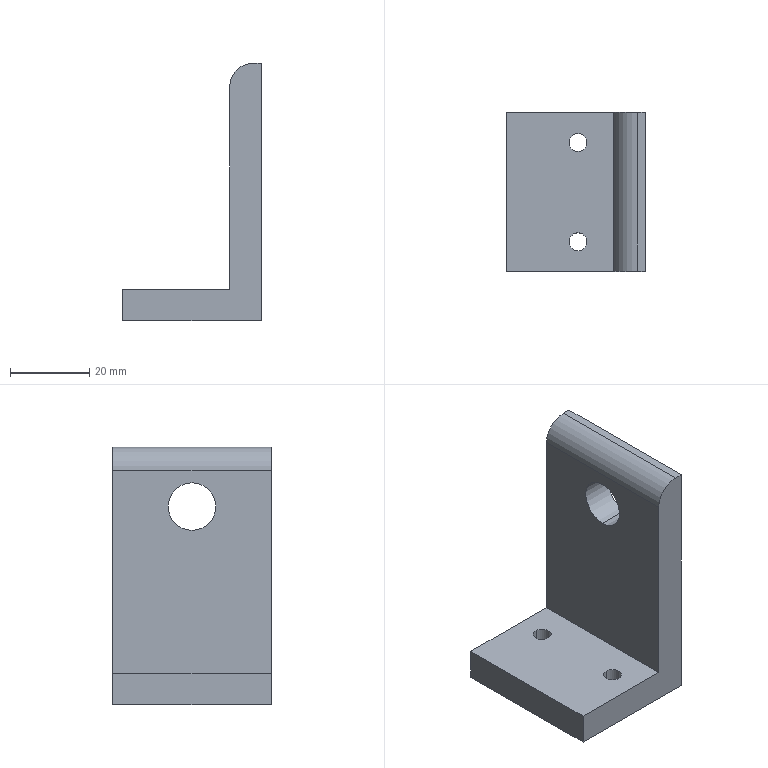Part | STEP file | Eyebolt mounting bracket-Part-1 | 1 solid | 15 faces | box 35 x 40 x 65 mm | volume 27972 mm3 | plane 8 | cylinder 7 | commonest cylinder face diameters 4.5 x4 12 x3
STEP:
#1=CARTESIAN_POINT('',(0.,0.,0.));
#2=DIRECTION('',(0.,0.,1.));
#3=DIRECTION('',(1.,0.,0.));
#4=AXIS2_PLACEMENT_3D('',#1,#2,#3);
#5=CARTESIAN_POINT('',(18.,5.25,8.));
#6=VERTEX_POINT('',#5);
#7=CARTESIAN_POINT('',(18.,5.25,0.));
#8=VERTEX_POINT('',#7);
#9=CARTESIAN_POINT('',(18.,5.25,8.));
#10=DIRECTION('',(0.,0.,-1.));
#11=VECTOR('',#10,1.);
#12=LINE('',#9,#11);
#13=CARTESIAN_POINT('',(18.,7.5,8.));
#14=DIRECTION('',(0.,0.,-1.));
#15=DIRECTION('',(0.,-1.,0.));
#16=AXIS2_PLACEMENT_3D('',#13,#14,#15);
#17=CYLINDRICAL_SURFACE('',#16,2.25);
#18=CARTESIAN_POINT('',(6.283,0.));
#19=DIRECTION('',(0.,1.));
#20=VECTOR('',#19,1.);
#21=LINE('',#18,#20);
#22=(GEOMETRIC_REPRESENTATION_CONTEXT(2)PARAMETRIC_REPRESENTATION_CONTEXT()REPRESENTATION_CONTEXT('',''));
#23=DEFINITIONAL_REPRESENTATION('',(#21),#22);
#24=PCURVE('',#17,#23);
#25=CARTESIAN_POINT('',(18.,7.5,8.));
#26=DIRECTION('',(0.,0.,-1.));
#27=DIRECTION('',(0.,-1.,0.));
#28=AXIS2_PLACEMENT_3D('',#25,#26,#27);
#29=CYLINDRICAL_SURFACE('',#28,2.25);
#30=CARTESIAN_POINT('',(0.,0.));
#31=DIRECTION('',(0.,1.));
#32=VECTOR('',#31,1.);
#33=LINE('',#30,#32);
#34=(GEOMETRIC_REPRESENTATION_CONTEXT(2)PARAMETRIC_REPRESENTATION_CONTEXT()REPRESENTATION_CONTEXT('',''));
#35=DEFINITIONAL_REPRESENTATION('',(#33),#34);
#36=PCURVE('',#29,#35);
#37=SURFACE_CURVE('',#12,(#24,#36),.PCURVE_S1.);
#38=EDGE_CURVE('',#6,#8,#37,.T.);
#39=ORIENTED_EDGE('',*,*,#38,.T.);
#40=CARTESIAN_POINT('',(18.,9.75,0.));
#41=VERTEX_POINT('',#40);
#42=CARTESIAN_POINT('',(18.,7.5,0.));
#43=DIRECTION('',(0.,0.,1.));
#44=DIRECTION('',(0.,1.,0.));
#45=AXIS2_PLACEMENT_3D('',#42,#43,#44);
#46=CIRCLE('',#45,2.25);
#47=CARTESIAN_POINT('',(9.425,8.));
#48=DIRECTION('',(-1.,0.));
#49=VECTOR('',#48,1.);
#50=LINE('',#47,#49);
#51=(GEOMETRIC_REPRESENTATION_CONTEXT(2)PARAMETRIC_REPRESENTATION_CONTEXT()REPRESENTATION_CONTEXT('',''));
#52=DEFINITIONAL_REPRESENTATION('',(#50),#51);
#53=PCURVE('',#17,#52);
#54=CARTESIAN_POINT('',(0.,0.,0.));
#55=DIRECTION('',(0.,0.,1.));
#56=DIRECTION('',(-1.,0.,0.));
#57=AXIS2_PLACEMENT_3D('',#54,#55,#56);
#58=PLANE('',#57);
#59=CARTESIAN_POINT('',(-18.,-7.5));
#60=DIRECTION('',(0.,-1.));
#61=AXIS2_PLACEMENT_2D('',#59,#60);
#62=CIRCLE('',#61,2.25);
#63=(GEOMETRIC_REPRESENTATION_CONTEXT(2)PARAMETRIC_REPRESENTATION_CONTEXT()REPRESENTATION_CONTEXT('',''));
#64=DEFINITIONAL_REPRESENTATION('',(#62),#63);
#65=PCURVE('',#58,#64);
#66=SURFACE_CURVE('',#46,(#53,#65),.PCURVE_S1.);
#67=EDGE_CURVE('',#8,#41,#66,.T.);
#68=ORIENTED_EDGE('',*,*,#67,.T.);
#69=CARTESIAN_POINT('',(18.,9.75,8.));
#70=VERTEX_POINT('',#69);
#71=CARTESIAN_POINT('',(18.,9.75,8.));
#72=DIRECTION('',(0.,0.,-1.));
#73=VECTOR('',#72,1.);
#74=LINE('',#71,#73);
#75=CARTESIAN_POINT('',(3.142,0.));
#76=DIRECTION('',(0.,1.));
#77=VECTOR('',#76,1.);
#78=LINE('',#75,#77);
#79=(GEOMETRIC_REPRESENTATION_CONTEXT(2)PARAMETRIC_REPRESENTATION_CONTEXT()REPRESENTATION_CONTEXT('',''));
#80=DEFINITIONAL_REPRESENTATION('',(#78),#79);
#81=PCURVE('',#17,#80);
#82=CARTESIAN_POINT('',(3.142,0.));
#83=DIRECTION('',(0.,1.));
#84=VECTOR('',#83,1.);
#85=LINE('',#82,#84);
#86=(GEOMETRIC_REPRESENTATION_CONTEXT(2)PARAMETRIC_REPRESENTATION_CONTEXT()REPRESENTATION_CONTEXT('',''));
#87=DEFINITIONAL_REPRESENTATION('',(#85),#86);
#88=PCURVE('',#29,#87);
#89=SURFACE_CURVE('',#74,(#81,#88),.PCURVE_S1.);
#90=EDGE_CURVE('',#70,#41,#89,.T.);
#91=ORIENTED_EDGE('',*,*,#90,.F.);
#92=CARTESIAN_POINT('',(18.,7.5,8.));
#93=DIRECTION('',(0.,0.,-1.));
#94=DIRECTION('',(0.,-1.,0.));
#95=AXIS2_PLACEMENT_3D('',#92,#93,#94);
#96=CIRCLE('',#95,2.25);
#97=CARTESIAN_POINT('',(0.,0.));
#98=DIRECTION('',(1.,0.));
#99=VECTOR('',#98,1.);
#100=LINE('',#97,#99);
#101=(GEOMETRIC_REPRESENTATION_CONTEXT(2)PARAMETRIC_REPRESENTATION_CONTEXT()REPRESENTATION_CONTEXT('',''));
#102=DEFINITIONAL_REPRESENTATION('',(#100),#101);
#103=PCURVE('',#17,#102);
#104=CARTESIAN_POINT('',(27.,0.,8.));
#105=DIRECTION('',(0.,0.,-1.));
#106=DIRECTION('',(1.,0.,0.));
#107=AXIS2_PLACEMENT_3D('',#104,#105,#106);
#108=PLANE('',#107);
#109=CARTESIAN_POINT('',(-9.,-7.5));
#110=DIRECTION('',(0.,1.));
#111=AXIS2_PLACEMENT_2D('',#109,#110);
#112=CIRCLE('',#111,2.25);
#113=(GEOMETRIC_REPRESENTATION_CONTEXT(2)PARAMETRIC_REPRESENTATION_CONTEXT()REPRESENTATION_CONTEXT('',''));
#114=DEFINITIONAL_REPRESENTATION('',(#112),#113);
#115=PCURVE('',#108,#114);
#116=SURFACE_CURVE('',#96,(#103,#115),.PCURVE_S1.);
#117=EDGE_CURVE('',#70,#6,#116,.T.);
#118=ORIENTED_EDGE('',*,*,#117,.T.);
#119=EDGE_LOOP('',(#39,#68,#91,#118));
#120=FACE_BOUND('',#119,.F.);
#121=ADVANCED_FACE('',(#120),#17,.F.);
#122=CARTESIAN_POINT('',(18.,30.25,8.));
#123=VERTEX_POINT('',#122);
#124=CARTESIAN_POINT('',(18.,30.25,0.));
#125=VERTEX_POINT('',#124);
#126=CARTESIAN_POINT('',(18.,30.25,8.));
#127=DIRECTION('',(0.,0.,-1.));
#128=VECTOR('',#127,1.);
#129=LINE('',#126,#128);
#130=CARTESIAN_POINT('',(18.,32.5,8.));
#131=DIRECTION('',(0.,0.,-1.));
#132=DIRECTION('',(0.,-1.,0.));
#133=AXIS2_PLACEMENT_3D('',#130,#131,#132);
#134=CYLINDRICAL_SURFACE('',#133,2.25);
#135=CARTESIAN_POINT('',(6.283,0.));
#136=DIRECTION('',(0.,1.));
#137=VECTOR('',#136,1.);
#138=LINE('',#135,#137);
#139=(GEOMETRIC_REPRESENTATION_CONTEXT(2)PARAMETRIC_REPRESENTATION_CONTEXT()REPRESENTATION_CONTEXT('',''));
#140=DEFINITIONAL_REPRESENTATION('',(#138),#139);
#141=PCURVE('',#134,#140);
#142=CARTESIAN_POINT('',(18.,32.5,8.));
#143=DIRECTION('',(0.,0.,-1.));
#144=DIRECTION('',(0.,-1.,0.));
#145=AXIS2_PLACEMENT_3D('',#142,#143,#144);
#146=CYLINDRICAL_SURFACE('',#145,2.25);
#147=CARTESIAN_POINT('',(0.,0.));
#148=DIRECTION('',(0.,1.));
#149=VECTOR('',#148,1.);
#150=LINE('',#147,#149);
#151=(GEOMETRIC_REPRESENTATION_CONTEXT(2)PARAMETRIC_REPRESENTATION_CONTEXT()REPRESENTATION_CONTEXT('',''));
#152=DEFINITIONAL_REPRESENTATION('',(#150),#151);
#153=PCURVE('',#146,#152);
#154=SURFACE_CURVE('',#129,(#141,#153),.PCURVE_S1.);
#155=EDGE_CURVE('',#123,#125,#154,.T.);
#156=ORIENTED_EDGE('',*,*,#155,.T.);
#157=CARTESIAN_POINT('',(18.,34.75,0.));
#158=VERTEX_POINT('',#157);
#159=CARTESIAN_POINT('',(18.,32.5,0.));
#160=DIRECTION('',(0.,0.,1.));
#161=DIRECTION('',(0.,1.,0.));
#162=AXIS2_PLACEMENT_3D('',#159,#160,#161);
#163=CIRCLE('',#162,2.25);
#164=CARTESIAN_POINT('',(9.425,8.));
#165=DIRECTION('',(-1.,0.));
#166=VECTOR('',#165,1.);
#167=LINE('',#164,#166);
#168=(GEOMETRIC_REPRESENTATION_CONTEXT(2)PARAMETRIC_REPRESENTATION_CONTEXT()REPRESENTATION_CONTEXT('',''));
#169=DEFINITIONAL_REPRESENTATION('',(#167),#168);
#170=PCURVE('',#134,#169);
#171=CARTESIAN_POINT('',(-18.,-32.5));
#172=DIRECTION('',(0.,-1.));
#173=AXIS2_PLACEMENT_2D('',#171,#172);
#174=CIRCLE('',#173,2.25);
#175=(GEOMETRIC_REPRESENTATION_CONTEXT(2)PARAMETRIC_REPRESENTATION_CONTEXT()REPRESENTATION_CONTEXT('',''));
#176=DEFINITIONAL_REPRESENTATION('',(#174),#175);
#177=PCURVE('',#58,#176);
#178=SURFACE_CURVE('',#163,(#170,#177),.PCURVE_S1.);
#179=EDGE_CURVE('',#125,#158,#178,.T.);
#180=ORIENTED_EDGE('',*,*,#179,.T.);
#181=CARTESIAN_POINT('',(18.,34.75,8.));
#182=VERTEX_POINT('',#181);
#183=CARTESIAN_POINT('',(18.,34.75,8.));
#184=DIRECTION('',(0.,0.,-1.));
#185=VECTOR('',#184,1.);
#186=LINE('',#183,#185);
#187=CARTESIAN_POINT('',(3.142,0.));
#188=DIRECTION('',(0.,1.));
#189=VECTOR('',#188,1.);
#190=LINE('',#187,#189);
#191=(GEOMETRIC_REPRESENTATION_CONTEXT(2)PARAMETRIC_REPRESENTATION_CONTEXT()REPRESENTATION_CONTEXT('',''));
#192=DEFINITIONAL_REPRESENTATION('',(#190),#191);
#193=PCURVE('',#134,#192);
#194=CARTESIAN_POINT('',(3.142,0.));
#195=DIRECTION('',(0.,1.));
#196=VECTOR('',#195,1.);
#197=LINE('',#194,#196);
#198=(GEOMETRIC_REPRESENTATION_CONTEXT(2)PARAMETRIC_REPRESENTATION_CONTEXT()REPRESENTATION_CONTEXT('',''));
#199=DEFINITIONAL_REPRESENTATION('',(#197),#198);
#200=PCURVE('',#146,#199);
#201=SURFACE_CURVE('',#186,(#193,#200),.PCURVE_S1.);
#202=EDGE_CURVE('',#182,#158,#201,.T.);
#203=ORIENTED_EDGE('',*,*,#202,.F.);
#204=CARTESIAN_POINT('',(18.,32.5,8.));
#205=DIRECTION('',(0.,0.,-1.));
#206=DIRECTION('',(0.,-1.,0.));
#207=AXIS2_PLACEMENT_3D('',#204,#205,#206);
#208=CIRCLE('',#207,2.25);
#209=CARTESIAN_POINT('',(0.,0.));
#210=DIRECTION('',(1.,0.));
#211=VECTOR('',#210,1.);
#212=LINE('',#209,#211);
#213=(GEOMETRIC_REPRESENTATION_CONTEXT(2)PARAMETRIC_REPRESENTATION_CONTEXT()REPRESENTATION_CONTEXT('',''));
#214=DEFINITIONAL_REPRESENTATION('',(#212),#213);
#215=PCURVE('',#134,#214);
#216=CARTESIAN_POINT('',(-9.,-32.5));
#217=DIRECTION('',(0.,1.));
#218=AXIS2_PLACEMENT_2D('',#216,#217);
#219=CIRCLE('',#218,2.25);
#220=(GEOMETRIC_REPRESENTATION_CONTEXT(2)PARAMETRIC_REPRESENTATION_CONTEXT()REPRESENTATION_CONTEXT('',''));
#221=DEFINITIONAL_REPRESENTATION('',(#219),#220);
#222=PCURVE('',#108,#221);
#223=SURFACE_CURVE('',#208,(#215,#222),.PCURVE_S1.);
#224=EDGE_CURVE('',#182,#123,#223,.T.);
#225=ORIENTED_EDGE('',*,*,#224,.T.);
#226=EDGE_LOOP('',(#156,#180,#203,#225));
#227=FACE_BOUND('',#226,.F.);
#228=ADVANCED_FACE('',(#227),#134,.F.);
#229=CARTESIAN_POINT('',(35.,20.,44.));
#230=VERTEX_POINT('',#229);
#231=CARTESIAN_POINT('',(27.,20.,44.));
#232=VERTEX_POINT('',#231);
#233=CARTESIAN_POINT('',(35.,20.,44.));
#234=DIRECTION('',(-1.,0.,0.));
#235=VECTOR('',#234,1.);
#236=LINE('',#233,#235);
#237=CARTESIAN_POINT('',(35.,20.,50.));
#238=DIRECTION('',(-1.,0.,0.));
#239=DIRECTION('',(0.,0.,-1.));
#240=AXIS2_PLACEMENT_3D('',#237,#238,#239);
#241=CYLINDRICAL_SURFACE('',#240,6.);
#242=CARTESIAN_POINT('',(6.283,0.));
#243=DIRECTION('',(0.,1.));
#244=VECTOR('',#243,1.);
#245=LINE('',#242,#244);
#246=(GEOMETRIC_REPRESENTATION_CONTEXT(2)PARAMETRIC_REPRESENTATION_CONTEXT()REPRESENTATION_CONTEXT('',''));
#247=DEFINITIONAL_REPRESENTATION('',(#245),#246);
#248=PCURVE('',#241,#247);
#249=CARTESIAN_POINT('',(35.,20.,50.));
#250=DIRECTION('',(-1.,0.,0.));
#251=DIRECTION('',(0.,0.,-1.));
#252=AXIS2_PLACEMENT_3D('',#249,#250,#251);
#253=CYLINDRICAL_SURFACE('',#252,6.);
#254=CARTESIAN_POINT('',(0.,0.));
#255=DIRECTION('',(0.,1.));
#256=VECTOR('',#255,1.);
#257=LINE('',#254,#256);
#258=(GEOMETRIC_REPRESENTATION_CONTEXT(2)PARAMETRIC_REPRESENTATION_CONTEXT()REPRESENTATION_CONTEXT('',''));
#259=DEFINITIONAL_REPRESENTATION('',(#257),#258);
#260=PCURVE('',#253,#259);
#261=SURFACE_CURVE('',#236,(#248,#260),.PCURVE_S1.);
#262=EDGE_CURVE('',#230,#232,#261,.T.);
#263=ORIENTED_EDGE('',*,*,#262,.T.);
#264=CARTESIAN_POINT('',(27.,20.,56.));
#265=VERTEX_POINT('',#264);
#266=CARTESIAN_POINT('',(27.,20.,50.));
#267=DIRECTION('',(1.,0.,0.));
#268=DIRECTION('',(0.,0.,1.));
#269=AXIS2_PLACEMENT_3D('',#266,#267,#268);
#270=CIRCLE('',#269,6.);
#271=CARTESIAN_POINT('',(9.425,8.));
#272=DIRECTION('',(-1.,0.));
#273=VECTOR('',#272,1.);
#274=LINE('',#271,#273);
#275=(GEOMETRIC_REPRESENTATION_CONTEXT(2)PARAMETRIC_REPRESENTATION_CONTEXT()REPRESENTATION_CONTEXT('',''));
#276=DEFINITIONAL_REPRESENTATION('',(#274),#275);
#277=PCURVE('',#241,#276);
#278=CARTESIAN_POINT('',(27.,0.,59.));
#279=DIRECTION('',(1.,0.,0.));
#280=DIRECTION('',(0.,0.,1.));
#281=AXIS2_PLACEMENT_3D('',#278,#279,#280);
#282=PLANE('',#281);
#283=CARTESIAN_POINT('',(-9.,-20.));
#284=DIRECTION('',(1.,0.));
#285=AXIS2_PLACEMENT_2D('',#283,#284);
#286=CIRCLE('',#285,6.);
#287=(GEOMETRIC_REPRESENTATION_CONTEXT(2)PARAMETRIC_REPRESENTATION_CONTEXT()REPRESENTATION_CONTEXT('',''));
#288=DEFINITIONAL_REPRESENTATION('',(#286),#287);
#289=PCURVE('',#282,#288);
#290=SURFACE_CURVE('',#270,(#277,#289),.PCURVE_S1.);
#291=EDGE_CURVE('',#232,#265,#290,.T.);
#292=ORIENTED_EDGE('',*,*,#291,.T.);
#293=CARTESIAN_POINT('',(35.,20.,56.));
#294=VERTEX_POINT('',#293);
#295=CARTESIAN_POINT('',(35.,20.,56.));
#296=DIRECTION('',(-1.,0.,0.));
#297=VECTOR('',#296,1.);
#298=LINE('',#295,#297);
#299=CARTESIAN_POINT('',(3.142,0.));
#300=DIRECTION('',(0.,1.));
#301=VECTOR('',#300,1.);
#302=LINE('',#299,#301);
#303=(GEOMETRIC_REPRESENTATION_CONTEXT(2)PARAMETRIC_REPRESENTATION_CONTEXT()REPRESENTATION_CONTEXT('',''));
#304=DEFINITIONAL_REPRESENTATION('',(#302),#303);
#305=PCURVE('',#241,#304);
#306=CARTESIAN_POINT('',(3.142,0.));
#307=DIRECTION('',(0.,1.));
#308=VECTOR('',#307,1.);
#309=LINE('',#306,#308);
#310=(GEOMETRIC_REPRESENTATION_CONTEXT(2)PARAMETRIC_REPRESENTATION_CONTEXT()REPRESENTATION_CONTEXT('',''));
#311=DEFINITIONAL_REPRESENTATION('',(#309),#310);
#312=PCURVE('',#253,#311);
#313=SURFACE_CURVE('',#298,(#305,#312),.PCURVE_S1.);
#314=EDGE_CURVE('',#294,#265,#313,.T.);
#315=ORIENTED_EDGE('',*,*,#314,.F.);
#316=CARTESIAN_POINT('',(35.,20.,50.));
#317=DIRECTION('',(-1.,0.,0.));
#318=DIRECTION('',(0.,0.,-1.));
#319=AXIS2_PLACEMENT_3D('',#316,#317,#318);
#320=CIRCLE('',#319,6.);
#321=CARTESIAN_POINT('',(0.,0.));
#322=DIRECTION('',(1.,0.));
#323=VECTOR('',#322,1.);
#324=LINE('',#321,#323);
#325=(GEOMETRIC_REPRESENTATION_CONTEXT(2)PARAMETRIC_REPRESENTATION_CONTEXT()REPRESENTATION_CONTEXT('',''));
#326=DEFINITIONAL_REPRESENTATION('',(#324),#325);
#327=PCURVE('',#241,#326);
#328=CARTESIAN_POINT('',(35.,0.,0.));
#329=DIRECTION('',(-1.,0.,0.));
#330=DIRECTION('',(0.,0.,-1.));
#331=AXIS2_PLACEMENT_3D('',#328,#329,#330);
#332=PLANE('',#331);
#333=CARTESIAN_POINT('',(-50.,-20.));
#334=DIRECTION('',(1.,0.));
#335=AXIS2_PLACEMENT_2D('',#333,#334);
#336=CIRCLE('',#335,6.);
#337=(GEOMETRIC_REPRESENTATION_CONTEXT(2)PARAMETRIC_REPRESENTATION_CONTEXT()REPRESENTATION_CONTEXT('',''));
#338=DEFINITIONAL_REPRESENTATION('',(#336),#337);
#339=PCURVE('',#332,#338);
#340=SURFACE_CURVE('',#320,(#327,#339),.PCURVE_S1.);
#341=EDGE_CURVE('',#294,#230,#340,.T.);
#342=ORIENTED_EDGE('',*,*,#341,.T.);
#343=EDGE_LOOP('',(#263,#292,#315,#342));
#344=FACE_BOUND('',#343,.F.);
#345=ADVANCED_FACE('',(#344),#241,.F.);
#346=ORIENTED_EDGE('',*,*,#67,.T.);
#347=CARTESIAN_POINT('',(18.,7.5,0.));
#348=DIRECTION('',(0.,0.,1.));
#349=DIRECTION('',(0.,1.,0.));
#350=AXIS2_PLACEMENT_3D('',#347,#348,#349);
#351=CIRCLE('',#350,2.25);
#352=CARTESIAN_POINT('',(-18.,-7.5));
#353=DIRECTION('',(0.,-1.));
#354=AXIS2_PLACEMENT_2D('',#352,#353);
#355=CIRCLE('',#354,2.25);
#356=(GEOMETRIC_REPRESENTATION_CONTEXT(2)PARAMETRIC_REPRESENTATION_CONTEXT()REPRESENTATION_CONTEXT('',''));
#357=DEFINITIONAL_REPRESENTATION('',(#355),#356);
#358=PCURVE('',#58,#357);
#359=CARTESIAN_POINT('',(3.142,8.));
#360=DIRECTION('',(-1.,0.));
#361=VECTOR('',#360,1.);
#362=LINE('',#359,#361);
#363=(GEOMETRIC_REPRESENTATION_CONTEXT(2)PARAMETRIC_REPRESENTATION_CONTEXT()REPRESENTATION_CONTEXT('',''));
#364=DEFINITIONAL_REPRESENTATION('',(#362),#363);
#365=PCURVE('',#29,#364);
#366=SURFACE_CURVE('',#351,(#358,#365),.PCURVE_S1.);
#367=EDGE_CURVE('',#41,#8,#366,.T.);
#368=ORIENTED_EDGE('',*,*,#367,.T.);
#369=EDGE_LOOP('',(#346,#368));
#370=FACE_BOUND('',#369,.T.);
#371=ORIENTED_EDGE('',*,*,#179,.T.);
#372=CARTESIAN_POINT('',(18.,32.5,0.));
#373=DIRECTION('',(0.,0.,1.));
#374=DIRECTION('',(0.,1.,0.));
#375=AXIS2_PLACEMENT_3D('',#372,#373,#374);
#376=CIRCLE('',#375,2.25);
#377=CARTESIAN_POINT('',(-18.,-32.5));
#378=DIRECTION('',(0.,-1.));
#379=AXIS2_PLACEMENT_2D('',#377,#378);
#380=CIRCLE('',#379,2.25);
#381=(GEOMETRIC_REPRESENTATION_CONTEXT(2)PARAMETRIC_REPRESENTATION_CONTEXT()REPRESENTATION_CONTEXT('',''));
#382=DEFINITIONAL_REPRESENTATION('',(#380),#381);
#383=PCURVE('',#58,#382);
#384=CARTESIAN_POINT('',(3.142,8.));
#385=DIRECTION('',(-1.,0.));
#386=VECTOR('',#385,1.);
#387=LINE('',#384,#386);
#388=(GEOMETRIC_REPRESENTATION_CONTEXT(2)PARAMETRIC_REPRESENTATION_CONTEXT()REPRESENTATION_CONTEXT('',''));
#389=DEFINITIONAL_REPRESENTATION('',(#387),#388);
#390=PCURVE('',#146,#389);
#391=SURFACE_CURVE('',#376,(#383,#390),.PCURVE_S1.);
#392=EDGE_CURVE('',#158,#125,#391,.T.);
#393=ORIENTED_EDGE('',*,*,#392,.T.);
#394=EDGE_LOOP('',(#371,#393));
#395=FACE_BOUND('',#394,.T.);
#396=CARTESIAN_POINT('',(0.,40.,0.));
#397=VERTEX_POINT('',#396);
#398=CARTESIAN_POINT('',(35.,40.,0.));
#399=VERTEX_POINT('',#398);
#400=CARTESIAN_POINT('',(0.,40.,0.));
#401=DIRECTION('',(1.,0.,0.));
#402=VECTOR('',#401,1.);
#403=LINE('',#400,#402);
#404=CARTESIAN_POINT('',(0.,-40.));
#405=DIRECTION('',(-1.,0.));
#406=VECTOR('',#405,1.);
#407=LINE('',#404,#406);
#408=(GEOMETRIC_REPRESENTATION_CONTEXT(2)PARAMETRIC_REPRESENTATION_CONTEXT()REPRESENTATION_CONTEXT('',''));
#409=DEFINITIONAL_REPRESENTATION('',(#407),#408);
#410=PCURVE('',#58,#409);
#411=CARTESIAN_POINT('',(33.,40.,59.));
#412=DIRECTION('',(0.,-1.,0.));
#413=DIRECTION('',(0.,0.,1.));
#414=AXIS2_PLACEMENT_3D('',#411,#412,#413);
#415=PLANE('',#414);
#416=CARTESIAN_POINT('',(-59.,33.));
#417=DIRECTION('',(0.,-1.));
#418=VECTOR('',#417,1.);
#419=LINE('',#416,#418);
#420=(GEOMETRIC_REPRESENTATION_CONTEXT(2)PARAMETRIC_REPRESENTATION_CONTEXT()REPRESENTATION_CONTEXT('',''));
#421=DEFINITIONAL_REPRESENTATION('',(#419),#420);
#422=PCURVE('',#415,#421);
#423=SURFACE_CURVE('',#403,(#410,#422),.PCURVE_S1.);
#424=EDGE_CURVE('',#397,#399,#423,.T.);
#425=ORIENTED_EDGE('',*,*,#424,.T.);
#426=CARTESIAN_POINT('',(35.,0.,0.));
#427=VERTEX_POINT('',#426);
#428=CARTESIAN_POINT('',(35.,0.,0.));
#429=DIRECTION('',(0.,1.,0.));
#430=VECTOR('',#429,1.);
#431=LINE('',#428,#430);
#432=CARTESIAN_POINT('',(-35.,0.));
#433=DIRECTION('',(0.,-1.));
#434=VECTOR('',#433,1.);
#435=LINE('',#432,#434);
#436=(GEOMETRIC_REPRESENTATION_CONTEXT(2)PARAMETRIC_REPRESENTATION_CONTEXT()REPRESENTATION_CONTEXT('',''));
#437=DEFINITIONAL_REPRESENTATION('',(#435),#436);
#438=PCURVE('',#58,#437);
#439=CARTESIAN_POINT('',(0.,0.));
#440=DIRECTION('',(0.,-1.));
#441=VECTOR('',#440,1.);
#442=LINE('',#439,#441);
#443=(GEOMETRIC_REPRESENTATION_CONTEXT(2)PARAMETRIC_REPRESENTATION_CONTEXT()REPRESENTATION_CONTEXT('',''));
#444=DEFINITIONAL_REPRESENTATION('',(#442),#443);
#445=PCURVE('',#332,#444);
#446=SURFACE_CURVE('',#431,(#438,#445),.PCURVE_S1.);
#447=EDGE_CURVE('',#427,#399,#446,.T.);
#448=ORIENTED_EDGE('',*,*,#447,.F.);
#449=CARTESIAN_POINT('',(0.,0.,0.));
#450=VERTEX_POINT('',#449);
#451=CARTESIAN_POINT('',(0.,0.,0.));
#452=DIRECTION('',(1.,0.,0.));
#453=VECTOR('',#452,1.);
#454=LINE('',#451,#453);
#455=CARTESIAN_POINT('',(0.,0.));
#456=DIRECTION('',(-1.,0.));
#457=VECTOR('',#456,1.);
#458=LINE('',#455,#457);
#459=(GEOMETRIC_REPRESENTATION_CONTEXT(2)PARAMETRIC_REPRESENTATION_CONTEXT()REPRESENTATION_CONTEXT('',''));
#460=DEFINITIONAL_REPRESENTATION('',(#458),#459);
#461=PCURVE('',#58,#460);
#462=CARTESIAN_POINT('',(33.,0.,59.));
#463=DIRECTION('',(0.,-1.,0.));
#464=DIRECTION('',(0.,0.,1.));
#465=AXIS2_PLACEMENT_3D('',#462,#463,#464);
#466=PLANE('',#465);
#467=CARTESIAN_POINT('',(-59.,33.));
#468=DIRECTION('',(0.,-1.));
#469=VECTOR('',#468,1.);
#470=LINE('',#467,#469);
#471=(GEOMETRIC_REPRESENTATION_CONTEXT(2)PARAMETRIC_REPRESENTATION_CONTEXT()REPRESENTATION_CONTEXT('',''));
#472=DEFINITIONAL_REPRESENTATION('',(#470),#471);
#473=PCURVE('',#466,#472);
#474=SURFACE_CURVE('',#454,(#461,#473),.PCURVE_S1.);
#475=EDGE_CURVE('',#450,#427,#474,.T.);
#476=ORIENTED_EDGE('',*,*,#475,.F.);
#477=CARTESIAN_POINT('',(0.,0.,0.));
#478=DIRECTION('',(0.,1.,0.));
#479=VECTOR('',#478,1.);
#480=LINE('',#477,#479);
#481=CARTESIAN_POINT('',(0.,0.));
#482=DIRECTION('',(0.,-1.));
#483=VECTOR('',#482,1.);
#484=LINE('',#481,#483);
#485=(GEOMETRIC_REPRESENTATION_CONTEXT(2)PARAMETRIC_REPRESENTATION_CONTEXT()REPRESENTATION_CONTEXT('',''));
#486=DEFINITIONAL_REPRESENTATION('',(#484),#485);
#487=PCURVE('',#58,#486);
#488=CARTESIAN_POINT('',(0.,0.,8.));
#489=DIRECTION('',(1.,0.,0.));
#490=DIRECTION('',(0.,1.,0.));
#491=AXIS2_PLACEMENT_3D('',#488,#489,#490);
#492=PLANE('',#491);
#493=CARTESIAN_POINT('',(0.,-8.));
#494=DIRECTION('',(1.,0.));
#495=VECTOR('',#494,1.);
#496=LINE('',#493,#495);
#497=(GEOMETRIC_REPRESENTATION_CONTEXT(2)PARAMETRIC_REPRESENTATION_CONTEXT()REPRESENTATION_CONTEXT('',''));
#498=DEFINITIONAL_REPRESENTATION('',(#496),#497);
#499=PCURVE('',#492,#498);
#500=SURFACE_CURVE('',#480,(#487,#499),.PCURVE_S1.);
#501=EDGE_CURVE('',#450,#397,#500,.T.);
#502=ORIENTED_EDGE('',*,*,#501,.T.);
#503=EDGE_LOOP('',(#425,#448,#476,#502));
#504=FACE_BOUND('',#503,.T.);
#505=ADVANCED_FACE('',(#370,#395,#504),#58,.F.);
#506=CARTESIAN_POINT('',(35.,20.,50.));
#507=DIRECTION('',(-1.,0.,0.));
#508=DIRECTION('',(0.,0.,-1.));
#509=AXIS2_PLACEMENT_3D('',#506,#507,#508);
#510=CIRCLE('',#509,6.);
#511=CARTESIAN_POINT('',(-50.,-20.));
#512=DIRECTION('',(1.,0.));
#513=AXIS2_PLACEMENT_2D('',#511,#512);
#514=CIRCLE('',#513,6.);
#515=(GEOMETRIC_REPRESENTATION_CONTEXT(2)PARAMETRIC_REPRESENTATION_CONTEXT()REPRESENTATION_CONTEXT('',''));
#516=DEFINITIONAL_REPRESENTATION('',(#514),#515);
#517=PCURVE('',#332,#516);
#518=CARTESIAN_POINT('',(0.,0.));
#519=DIRECTION('',(1.,0.));
#520=VECTOR('',#519,1.);
#521=LINE('',#518,#520);
#522=(GEOMETRIC_REPRESENTATION_CONTEXT(2)PARAMETRIC_REPRESENTATION_CONTEXT()REPRESENTATION_CONTEXT('',''));
#523=DEFINITIONAL_REPRESENTATION('',(#521),#522);
#524=PCURVE('',#253,#523);
#525=SURFACE_CURVE('',#510,(#517,#524),.PCURVE_S1.);
#526=EDGE_CURVE('',#230,#294,#525,.T.);
#527=ORIENTED_EDGE('',*,*,#526,.T.);
#528=ORIENTED_EDGE('',*,*,#341,.T.);
#529=EDGE_LOOP('',(#527,#528));
#530=FACE_BOUND('',#529,.T.);
#531=CARTESIAN_POINT('',(35.,40.,65.));
#532=VERTEX_POINT('',#531);
#533=CARTESIAN_POINT('',(35.,40.,0.));
#534=DIRECTION('',(0.,0.,1.));
#535=VECTOR('',#534,1.);
#536=LINE('',#533,#535);
#537=CARTESIAN_POINT('',(0.,-40.));
#538=DIRECTION('',(-1.,0.));
#539=VECTOR('',#538,1.);
#540=LINE('',#537,#539);
#541=(GEOMETRIC_REPRESENTATION_CONTEXT(2)PARAMETRIC_REPRESENTATION_CONTEXT()REPRESENTATION_CONTEXT('',''));
#542=DEFINITIONAL_REPRESENTATION('',(#540),#541);
#543=PCURVE('',#332,#542);
#544=CARTESIAN_POINT('',(-59.,-2.));
#545=DIRECTION('',(1.,0.));
#546=VECTOR('',#545,1.);
#547=LINE('',#544,#546);
#548=(GEOMETRIC_REPRESENTATION_CONTEXT(2)PARAMETRIC_REPRESENTATION_CONTEXT()REPRESENTATION_CONTEXT('',''));
#549=DEFINITIONAL_REPRESENTATION('',(#547),#548);
#550=PCURVE('',#415,#549);
#551=SURFACE_CURVE('',#536,(#543,#550),.PCURVE_S1.);
#552=EDGE_CURVE('',#399,#532,#551,.T.);
#553=ORIENTED_EDGE('',*,*,#552,.T.);
#554=CARTESIAN_POINT('',(35.,0.,65.));
#555=VERTEX_POINT('',#554);
#556=CARTESIAN_POINT('',(35.,0.,65.));
#557=DIRECTION('',(0.,1.,0.));
#558=VECTOR('',#557,1.);
#559=LINE('',#556,#558);
#560=CARTESIAN_POINT('',(-65.,0.));
#561=DIRECTION('',(0.,-1.));
#562=VECTOR('',#561,1.);
#563=LINE('',#560,#562);
#564=(GEOMETRIC_REPRESENTATION_CONTEXT(2)PARAMETRIC_REPRESENTATION_CONTEXT()REPRESENTATION_CONTEXT('',''));
#565=DEFINITIONAL_REPRESENTATION('',(#563),#564);
#566=PCURVE('',#332,#565);
#567=CARTESIAN_POINT('',(35.,0.,65.));
#568=DIRECTION('',(0.,0.,-1.));
#569=DIRECTION('',(0.,-1.,0.));
#570=AXIS2_PLACEMENT_3D('',#567,#568,#569);
#571=PLANE('',#570);
#572=CARTESIAN_POINT('',(0.,0.));
#573=DIRECTION('',(-1.,0.));
#574=VECTOR('',#573,1.);
#575=LINE('',#572,#574);
#576=(GEOMETRIC_REPRESENTATION_CONTEXT(2)PARAMETRIC_REPRESENTATION_CONTEXT()REPRESENTATION_CONTEXT('',''));
#577=DEFINITIONAL_REPRESENTATION('',(#575),#576);
#578=PCURVE('',#571,#577);
#579=SURFACE_CURVE('',#559,(#566,#578),.PCURVE_S1.);
#580=EDGE_CURVE('',#555,#532,#579,.T.);
#581=ORIENTED_EDGE('',*,*,#580,.F.);
#582=CARTESIAN_POINT('',(35.,0.,0.));
#583=DIRECTION('',(0.,0.,1.));
#584=VECTOR('',#583,1.);
#585=LINE('',#582,#584);
#586=CARTESIAN_POINT('',(0.,0.));
#587=DIRECTION('',(-1.,0.));
#588=VECTOR('',#587,1.);
#589=LINE('',#586,#588);
#590=(GEOMETRIC_REPRESENTATION_CONTEXT(2)PARAMETRIC_REPRESENTATION_CONTEXT()REPRESENTATION_CONTEXT('',''));
#591=DEFINITIONAL_REPRESENTATION('',(#589),#590);
#592=PCURVE('',#332,#591);
#593=CARTESIAN_POINT('',(-59.,-2.));
#594=DIRECTION('',(1.,0.));
#595=VECTOR('',#594,1.);
#596=LINE('',#593,#595);
#597=(GEOMETRIC_REPRESENTATION_CONTEXT(2)PARAMETRIC_REPRESENTATION_CONTEXT()REPRESENTATION_CONTEXT('',''));
#598=DEFINITIONAL_REPRESENTATION('',(#596),#597);
#599=PCURVE('',#466,#598);
#600=SURFACE_CURVE('',#585,(#592,#599),.PCURVE_S1.);
#601=EDGE_CURVE('',#427,#555,#600,.T.);
#602=ORIENTED_EDGE('',*,*,#601,.F.);
#603=ORIENTED_EDGE('',*,*,#447,.T.);
#604=EDGE_LOOP('',(#553,#581,#602,#603));
#605=FACE_BOUND('',#604,.T.);
#606=ADVANCED_FACE('',(#530,#605),#332,.F.);
#607=CARTESIAN_POINT('',(33.,40.,65.));
#608=VERTEX_POINT('',#607);
#609=CARTESIAN_POINT('',(35.,40.,65.));
#610=DIRECTION('',(-1.,0.,0.));
#611=VECTOR('',#610,1.);
#612=LINE('',#609,#611);
#613=CARTESIAN_POINT('',(-40.,0.));
#614=DIRECTION('',(0.,1.));
#615=VECTOR('',#614,1.);
#616=LINE('',#613,#615);
#617=(GEOMETRIC_REPRESENTATION_CONTEXT(2)PARAMETRIC_REPRESENTATION_CONTEXT()REPRESENTATION_CONTEXT('',''));
#618=DEFINITIONAL_REPRESENTATION('',(#616),#617);
#619=PCURVE('',#571,#618);
#620=CARTESIAN_POINT('',(6.,-2.));
#621=DIRECTION('',(0.,1.));
#622=VECTOR('',#621,1.);
#623=LINE('',#620,#622);
#624=(GEOMETRIC_REPRESENTATION_CONTEXT(2)PARAMETRIC_REPRESENTATION_CONTEXT()REPRESENTATION_CONTEXT('',''));
#625=DEFINITIONAL_REPRESENTATION('',(#623),#624);
#626=PCURVE('',#415,#625);
#627=SURFACE_CURVE('',#612,(#619,#626),.PCURVE_S1.);
#628=EDGE_CURVE('',#532,#608,#627,.T.);
#629=ORIENTED_EDGE('',*,*,#628,.T.);
#630=CARTESIAN_POINT('',(33.,0.,65.));
#631=VERTEX_POINT('',#630);
#632=CARTESIAN_POINT('',(33.,0.,65.));
#633=DIRECTION('',(0.,1.,0.));
#634=VECTOR('',#633,1.);
#635=LINE('',#632,#634);
#636=CARTESIAN_POINT('',(0.,2.));
#637=DIRECTION('',(-1.,0.));
#638=VECTOR('',#637,1.);
#639=LINE('',#636,#638);
#640=(GEOMETRIC_REPRESENTATION_CONTEXT(2)PARAMETRIC_REPRESENTATION_CONTEXT()REPRESENTATION_CONTEXT('',''));
#641=DEFINITIONAL_REPRESENTATION('',(#639),#640);
#642=PCURVE('',#571,#641);
#643=CARTESIAN_POINT('',(33.,0.,59.));
#644=DIRECTION('',(0.,1.,0.));
#645=DIRECTION('',(0.,0.,-1.));
#646=AXIS2_PLACEMENT_3D('',#643,#644,#645);
#647=CYLINDRICAL_SURFACE('',#646,6.);
#648=CARTESIAN_POINT('',(3.142,0.));
#649=DIRECTION('',(0.,1.));
#650=VECTOR('',#649,1.);
#651=LINE('',#648,#650);
#652=(GEOMETRIC_REPRESENTATION_CONTEXT(2)PARAMETRIC_REPRESENTATION_CONTEXT()REPRESENTATION_CONTEXT('',''));
#653=DEFINITIONAL_REPRESENTATION('',(#651),#652);
#654=PCURVE('',#647,#653);
#655=SURFACE_CURVE('',#635,(#642,#654),.PCURVE_S1.);
#656=EDGE_CURVE('',#631,#608,#655,.T.);
#657=ORIENTED_EDGE('',*,*,#656,.F.);
#658=CARTESIAN_POINT('',(35.,0.,65.));
#659=DIRECTION('',(-1.,0.,0.));
#660=VECTOR('',#659,1.);
#661=LINE('',#658,#660);
#662=CARTESIAN_POINT('',(0.,0.));
#663=DIRECTION('',(0.,1.));
#664=VECTOR('',#663,1.);
#665=LINE('',#662,#664);
#666=(GEOMETRIC_REPRESENTATION_CONTEXT(2)PARAMETRIC_REPRESENTATION_CONTEXT()REPRESENTATION_CONTEXT('',''));
#667=DEFINITIONAL_REPRESENTATION('',(#665),#666);
#668=PCURVE('',#571,#667);
#669=CARTESIAN_POINT('',(6.,-2.));
#670=DIRECTION('',(0.,1.));
#671=VECTOR('',#670,1.);
#672=LINE('',#669,#671);
#673=(GEOMETRIC_REPRESENTATION_CONTEXT(2)PARAMETRIC_REPRESENTATION_CONTEXT()REPRESENTATION_CONTEXT('',''));
#674=DEFINITIONAL_REPRESENTATION('',(#672),#673);
#675=PCURVE('',#466,#674);
#676=SURFACE_CURVE('',#661,(#668,#675),.PCURVE_S1.);
#677=EDGE_CURVE('',#555,#631,#676,.T.);
#678=ORIENTED_EDGE('',*,*,#677,.F.);
#679=ORIENTED_EDGE('',*,*,#580,.T.);
#680=EDGE_LOOP('',(#629,#657,#678,#679));
#681=FACE_BOUND('',#680,.T.);
#682=ADVANCED_FACE('',(#681),#571,.F.);
#683=CARTESIAN_POINT('',(27.,40.,59.));
#684=VERTEX_POINT('',#683);
#685=CARTESIAN_POINT('',(33.,40.,59.));
#686=DIRECTION('',(0.,-1.,0.));
#687=DIRECTION('',(0.,0.,1.));
#688=AXIS2_PLACEMENT_3D('',#685,#686,#687);
#689=CIRCLE('',#688,6.);
#690=CARTESIAN_POINT('',(3.142,40.));
#691=DIRECTION('',(-1.,0.));
#692=VECTOR('',#691,1.);
#693=LINE('',#690,#692);
#694=(GEOMETRIC_REPRESENTATION_CONTEXT(2)PARAMETRIC_REPRESENTATION_CONTEXT()REPRESENTATION_CONTEXT('',''));
#695=DEFINITIONAL_REPRESENTATION('',(#693),#694);
#696=PCURVE('',#647,#695);
#697=CARTESIAN_POINT('',(0.,0.));
#698=DIRECTION('',(1.,0.));
#699=AXIS2_PLACEMENT_2D('',#697,#698);
#700=CIRCLE('',#699,6.);
#701=(GEOMETRIC_REPRESENTATION_CONTEXT(2)PARAMETRIC_REPRESENTATION_CONTEXT()REPRESENTATION_CONTEXT('',''));
#702=DEFINITIONAL_REPRESENTATION('',(#700),#701);
#703=PCURVE('',#415,#702);
#704=SURFACE_CURVE('',#689,(#696,#703),.PCURVE_S1.);
#705=EDGE_CURVE('',#608,#684,#704,.T.);
#706=ORIENTED_EDGE('',*,*,#705,.T.);
#707=CARTESIAN_POINT('',(27.,0.,59.));
#708=VERTEX_POINT('',#707);
#709=CARTESIAN_POINT('',(27.,0.,59.));
#710=DIRECTION('',(0.,1.,0.));
#711=VECTOR('',#710,1.);
#712=LINE('',#709,#711);
#713=CARTESIAN_POINT('',(1.571,0.));
#714=DIRECTION('',(0.,1.));
#715=VECTOR('',#714,1.);
#716=LINE('',#713,#715);
#717=(GEOMETRIC_REPRESENTATION_CONTEXT(2)PARAMETRIC_REPRESENTATION_CONTEXT()REPRESENTATION_CONTEXT('',''));
#718=DEFINITIONAL_REPRESENTATION('',(#716),#717);
#719=PCURVE('',#647,#718);
#720=CARTESIAN_POINT('',(0.,0.));
#721=DIRECTION('',(0.,-1.));
#722=VECTOR('',#721,1.);
#723=LINE('',#720,#722);
#724=(GEOMETRIC_REPRESENTATION_CONTEXT(2)PARAMETRIC_REPRESENTATION_CONTEXT()REPRESENTATION_CONTEXT('',''));
#725=DEFINITIONAL_REPRESENTATION('',(#723),#724);
#726=PCURVE('',#282,#725);
#727=SURFACE_CURVE('',#712,(#719,#726),.PCURVE_S1.);
#728=EDGE_CURVE('',#708,#684,#727,.T.);
#729=ORIENTED_EDGE('',*,*,#728,.F.);
#730=CARTESIAN_POINT('',(33.,0.,59.));
#731=DIRECTION('',(0.,-1.,0.));
#732=DIRECTION('',(0.,0.,1.));
#733=AXIS2_PLACEMENT_3D('',#730,#731,#732);
#734=CIRCLE('',#733,6.);
#735=CARTESIAN_POINT('',(3.142,0.));
#736=DIRECTION('',(-1.,0.));
#737=VECTOR('',#736,1.);
#738=LINE('',#735,#737);
#739=(GEOMETRIC_REPRESENTATION_CONTEXT(2)PARAMETRIC_REPRESENTATION_CONTEXT()REPRESENTATION_CONTEXT('',''));
#740=DEFINITIONAL_REPRESENTATION('',(#738),#739);
#741=PCURVE('',#647,#740);
#742=CARTESIAN_POINT('',(0.,0.));
#743=DIRECTION('',(1.,0.));
#744=AXIS2_PLACEMENT_2D('',#742,#743);
#745=CIRCLE('',#744,6.);
#746=(GEOMETRIC_REPRESENTATION_CONTEXT(2)PARAMETRIC_REPRESENTATION_CONTEXT()REPRESENTATION_CONTEXT('',''));
#747=DEFINITIONAL_REPRESENTATION('',(#745),#746);
#748=PCURVE('',#466,#747);
#749=SURFACE_CURVE('',#734,(#741,#748),.PCURVE_S1.);
#750=EDGE_CURVE('',#631,#708,#749,.T.);
#751=ORIENTED_EDGE('',*,*,#750,.F.);
#752=ORIENTED_EDGE('',*,*,#656,.T.);
#753=EDGE_LOOP('',(#706,#729,#751,#752));
#754=FACE_BOUND('',#753,.T.);
#755=ADVANCED_FACE('',(#754),#647,.T.);
#756=ORIENTED_EDGE('',*,*,#291,.T.);
#757=CARTESIAN_POINT('',(27.,20.,50.));
#758=DIRECTION('',(1.,0.,0.));
#759=DIRECTION('',(0.,0.,1.));
#760=AXIS2_PLACEMENT_3D('',#757,#758,#759);
#761=CIRCLE('',#760,6.);
#762=CARTESIAN_POINT('',(-9.,-20.));
#763=DIRECTION('',(1.,0.));
#764=AXIS2_PLACEMENT_2D('',#762,#763);
#765=CIRCLE('',#764,6.);
#766=(GEOMETRIC_REPRESENTATION_CONTEXT(2)PARAMETRIC_REPRESENTATION_CONTEXT()REPRESENTATION_CONTEXT('',''));
#767=DEFINITIONAL_REPRESENTATION('',(#765),#766);
#768=PCURVE('',#282,#767);
#769=CARTESIAN_POINT('',(3.142,8.));
#770=DIRECTION('',(-1.,0.));
#771=VECTOR('',#770,1.);
#772=LINE('',#769,#771);
#773=(GEOMETRIC_REPRESENTATION_CONTEXT(2)PARAMETRIC_REPRESENTATION_CONTEXT()REPRESENTATION_CONTEXT('',''));
#774=DEFINITIONAL_REPRESENTATION('',(#772),#773);
#775=PCURVE('',#253,#774);
#776=SURFACE_CURVE('',#761,(#768,#775),.PCURVE_S1.);
#777=EDGE_CURVE('',#265,#232,#776,.T.);
#778=ORIENTED_EDGE('',*,*,#777,.T.);
#779=EDGE_LOOP('',(#756,#778));
#780=FACE_BOUND('',#779,.T.);
#781=CARTESIAN_POINT('',(27.,40.,8.));
#782=VERTEX_POINT('',#781);
#783=CARTESIAN_POINT('',(27.,40.,59.));
#784=DIRECTION('',(0.,0.,-1.));
#785=VECTOR('',#784,1.);
#786=LINE('',#783,#785);
#787=CARTESIAN_POINT('',(0.,-40.));
#788=DIRECTION('',(-1.,0.));
#789=VECTOR('',#788,1.);
#790=LINE('',#787,#789);
#791=(GEOMETRIC_REPRESENTATION_CONTEXT(2)PARAMETRIC_REPRESENTATION_CONTEXT()REPRESENTATION_CONTEXT('',''));
#792=DEFINITIONAL_REPRESENTATION('',(#790),#791);
#793=PCURVE('',#282,#792);
#794=CARTESIAN_POINT('',(0.,6.));
#795=DIRECTION('',(-1.,0.));
#796=VECTOR('',#795,1.);
#797=LINE('',#794,#796);
#798=(GEOMETRIC_REPRESENTATION_CONTEXT(2)PARAMETRIC_REPRESENTATION_CONTEXT()REPRESENTATION_CONTEXT('',''));
#799=DEFINITIONAL_REPRESENTATION('',(#797),#798);
#800=PCURVE('',#415,#799);
#801=SURFACE_CURVE('',#786,(#793,#800),.PCURVE_S1.);
#802=EDGE_CURVE('',#684,#782,#801,.T.);
#803=ORIENTED_EDGE('',*,*,#802,.T.);
#804=CARTESIAN_POINT('',(27.,0.,8.));
#805=VERTEX_POINT('',#804);
#806=CARTESIAN_POINT('',(27.,0.,8.));
#807=DIRECTION('',(0.,1.,0.));
#808=VECTOR('',#807,1.);
#809=LINE('',#806,#808);
#810=CARTESIAN_POINT('',(-51.,0.));
#811=DIRECTION('',(0.,-1.));
#812=VECTOR('',#811,1.);
#813=LINE('',#810,#812);
#814=(GEOMETRIC_REPRESENTATION_CONTEXT(2)PARAMETRIC_REPRESENTATION_CONTEXT()REPRESENTATION_CONTEXT('',''));
#815=DEFINITIONAL_REPRESENTATION('',(#813),#814);
#816=PCURVE('',#282,#815);
#817=CARTESIAN_POINT('',(0.,0.));
#818=DIRECTION('',(0.,-1.));
#819=VECTOR('',#818,1.);
#820=LINE('',#817,#819);
#821=(GEOMETRIC_REPRESENTATION_CONTEXT(2)PARAMETRIC_REPRESENTATION_CONTEXT()REPRESENTATION_CONTEXT('',''));
#822=DEFINITIONAL_REPRESENTATION('',(#820),#821);
#823=PCURVE('',#108,#822);
#824=SURFACE_CURVE('',#809,(#816,#823),.PCURVE_S1.);
#825=EDGE_CURVE('',#805,#782,#824,.T.);
#826=ORIENTED_EDGE('',*,*,#825,.F.);
#827=CARTESIAN_POINT('',(27.,0.,59.));
#828=DIRECTION('',(0.,0.,-1.));
#829=VECTOR('',#828,1.);
#830=LINE('',#827,#829);
#831=CARTESIAN_POINT('',(0.,0.));
#832=DIRECTION('',(-1.,0.));
#833=VECTOR('',#832,1.);
#834=LINE('',#831,#833);
#835=(GEOMETRIC_REPRESENTATION_CONTEXT(2)PARAMETRIC_REPRESENTATION_CONTEXT()REPRESENTATION_CONTEXT('',''));
#836=DEFINITIONAL_REPRESENTATION('',(#834),#835);
#837=PCURVE('',#282,#836);
#838=CARTESIAN_POINT('',(0.,6.));
#839=DIRECTION('',(-1.,0.));
#840=VECTOR('',#839,1.);
#841=LINE('',#838,#840);
#842=(GEOMETRIC_REPRESENTATION_CONTEXT(2)PARAMETRIC_REPRESENTATION_CONTEXT()REPRESENTATION_CONTEXT('',''));
#843=DEFINITIONAL_REPRESENTATION('',(#841),#842);
#844=PCURVE('',#466,#843);
#845=SURFACE_CURVE('',#830,(#837,#844),.PCURVE_S1.);
#846=EDGE_CURVE('',#708,#805,#845,.T.);
#847=ORIENTED_EDGE('',*,*,#846,.F.);
#848=ORIENTED_EDGE('',*,*,#728,.T.);
#849=EDGE_LOOP('',(#803,#826,#847,#848));
#850=FACE_BOUND('',#849,.T.);
#851=ADVANCED_FACE('',(#780,#850),#282,.F.);
#852=CARTESIAN_POINT('',(18.,7.5,8.));
#853=DIRECTION('',(0.,0.,-1.));
#854=DIRECTION('',(0.,-1.,0.));
#855=AXIS2_PLACEMENT_3D('',#852,#853,#854);
#856=CIRCLE('',#855,2.25);
#857=CARTESIAN_POINT('',(-9.,-7.5));
#858=DIRECTION('',(0.,1.));
#859=AXIS2_PLACEMENT_2D('',#857,#858);
#860=CIRCLE('',#859,2.25);
#861=(GEOMETRIC_REPRESENTATION_CONTEXT(2)PARAMETRIC_REPRESENTATION_CONTEXT()REPRESENTATION_CONTEXT('',''));
#862=DEFINITIONAL_REPRESENTATION('',(#860),#861);
#863=PCURVE('',#108,#862);
#864=CARTESIAN_POINT('',(0.,0.));
#865=DIRECTION('',(1.,0.));
#866=VECTOR('',#865,1.);
#867=LINE('',#864,#866);
#868=(GEOMETRIC_REPRESENTATION_CONTEXT(2)PARAMETRIC_REPRESENTATION_CONTEXT()REPRESENTATION_CONTEXT('',''));
#869=DEFINITIONAL_REPRESENTATION('',(#867),#868);
#870=PCURVE('',#29,#869);
#871=SURFACE_CURVE('',#856,(#863,#870),.PCURVE_S1.);
#872=EDGE_CURVE('',#6,#70,#871,.T.);
#873=ORIENTED_EDGE('',*,*,#872,.T.);
#874=ORIENTED_EDGE('',*,*,#117,.T.);
#875=EDGE_LOOP('',(#873,#874));
#876=FACE_BOUND('',#875,.T.);
#877=CARTESIAN_POINT('',(18.,32.5,8.));
#878=DIRECTION('',(0.,0.,-1.));
#879=DIRECTION('',(0.,-1.,0.));
#880=AXIS2_PLACEMENT_3D('',#877,#878,#879);
#881=CIRCLE('',#880,2.25);
#882=CARTESIAN_POINT('',(-9.,-32.5));
#883=DIRECTION('',(0.,1.));
#884=AXIS2_PLACEMENT_2D('',#882,#883);
#885=CIRCLE('',#884,2.25);
#886=(GEOMETRIC_REPRESENTATION_CONTEXT(2)PARAMETRIC_REPRESENTATION_CONTEXT()REPRESENTATION_CONTEXT('',''));
#887=DEFINITIONAL_REPRESENTATION('',(#885),#886);
#888=PCURVE('',#108,#887);
#889=CARTESIAN_POINT('',(0.,0.));
#890=DIRECTION('',(1.,0.));
#891=VECTOR('',#890,1.);
#892=LINE('',#889,#891);
#893=(GEOMETRIC_REPRESENTATION_CONTEXT(2)PARAMETRIC_REPRESENTATION_CONTEXT()REPRESENTATION_CONTEXT('',''));
#894=DEFINITIONAL_REPRESENTATION('',(#892),#893);
#895=PCURVE('',#146,#894);
#896=SURFACE_CURVE('',#881,(#888,#895),.PCURVE_S1.);
#897=EDGE_CURVE('',#123,#182,#896,.T.);
#898=ORIENTED_EDGE('',*,*,#897,.T.);
#899=ORIENTED_EDGE('',*,*,#224,.T.);
#900=EDGE_LOOP('',(#898,#899));
#901=FACE_BOUND('',#900,.T.);
#902=CARTESIAN_POINT('',(0.,40.,8.));
#903=VERTEX_POINT('',#902);
#904=CARTESIAN_POINT('',(27.,40.,8.));
#905=DIRECTION('',(-1.,0.,0.));
#906=VECTOR('',#905,1.);
#907=LINE('',#904,#906);
#908=CARTESIAN_POINT('',(0.,-40.));
#909=DIRECTION('',(-1.,0.));
#910=VECTOR('',#909,1.);
#911=LINE('',#908,#910);
#912=(GEOMETRIC_REPRESENTATION_CONTEXT(2)PARAMETRIC_REPRESENTATION_CONTEXT()REPRESENTATION_CONTEXT('',''));
#913=DEFINITIONAL_REPRESENTATION('',(#911),#912);
#914=PCURVE('',#108,#913);
#915=CARTESIAN_POINT('',(-51.,6.));
#916=DIRECTION('',(0.,1.));
#917=VECTOR('',#916,1.);
#918=LINE('',#915,#917);
#919=(GEOMETRIC_REPRESENTATION_CONTEXT(2)PARAMETRIC_REPRESENTATION_CONTEXT()REPRESENTATION_CONTEXT('',''));
#920=DEFINITIONAL_REPRESENTATION('',(#918),#919);
#921=PCURVE('',#415,#920);
#922=SURFACE_CURVE('',#907,(#914,#921),.PCURVE_S1.);
#923=EDGE_CURVE('',#782,#903,#922,.T.);
#924=ORIENTED_EDGE('',*,*,#923,.T.);
#925=CARTESIAN_POINT('',(0.,0.,8.));
#926=VERTEX_POINT('',#925);
#927=CARTESIAN_POINT('',(0.,0.,8.));
#928=DIRECTION('',(0.,1.,0.));
#929=VECTOR('',#928,1.);
#930=LINE('',#927,#929);
#931=CARTESIAN_POINT('',(-27.,0.));
#932=DIRECTION('',(0.,-1.));
#933=VECTOR('',#932,1.);
#934=LINE('',#931,#933);
#935=(GEOMETRIC_REPRESENTATION_CONTEXT(2)PARAMETRIC_REPRESENTATION_CONTEXT()REPRESENTATION_CONTEXT('',''));
#936=DEFINITIONAL_REPRESENTATION('',(#934),#935);
#937=PCURVE('',#108,#936);
#938=CARTESIAN_POINT('',(0.,0.));
#939=DIRECTION('',(1.,0.));
#940=VECTOR('',#939,1.);
#941=LINE('',#938,#940);
#942=(GEOMETRIC_REPRESENTATION_CONTEXT(2)PARAMETRIC_REPRESENTATION_CONTEXT()REPRESENTATION_CONTEXT('',''));
#943=DEFINITIONAL_REPRESENTATION('',(#941),#942);
#944=PCURVE('',#492,#943);
#945=SURFACE_CURVE('',#930,(#937,#944),.PCURVE_S1.);
#946=EDGE_CURVE('',#926,#903,#945,.T.);
#947=ORIENTED_EDGE('',*,*,#946,.F.);
#948=CARTESIAN_POINT('',(27.,0.,8.));
#949=DIRECTION('',(-1.,0.,0.));
#950=VECTOR('',#949,1.);
#951=LINE('',#948,#950);
#952=CARTESIAN_POINT('',(0.,0.));
#953=DIRECTION('',(-1.,0.));
#954=VECTOR('',#953,1.);
#955=LINE('',#952,#954);
#956=(GEOMETRIC_REPRESENTATION_CONTEXT(2)PARAMETRIC_REPRESENTATION_CONTEXT()REPRESENTATION_CONTEXT('',''));
#957=DEFINITIONAL_REPRESENTATION('',(#955),#956);
#958=PCURVE('',#108,#957);
#959=CARTESIAN_POINT('',(-51.,6.));
#960=DIRECTION('',(0.,1.));
#961=VECTOR('',#960,1.);
#962=LINE('',#959,#961);
#963=(GEOMETRIC_REPRESENTATION_CONTEXT(2)PARAMETRIC_REPRESENTATION_CONTEXT()REPRESENTATION_CONTEXT('',''));
#964=DEFINITIONAL_REPRESENTATION('',(#962),#963);
#965=PCURVE('',#466,#964);
#966=SURFACE_CURVE('',#951,(#958,#965),.PCURVE_S1.);
#967=EDGE_CURVE('',#805,#926,#966,.T.);
#968=ORIENTED_EDGE('',*,*,#967,.F.);
#969=ORIENTED_EDGE('',*,*,#825,.T.);
#970=EDGE_LOOP('',(#924,#947,#968,#969));
#971=FACE_BOUND('',#970,.T.);
#972=ADVANCED_FACE('',(#876,#901,#971),#108,.F.);
#973=CARTESIAN_POINT('',(0.,40.,8.));
#974=DIRECTION('',(0.,0.,-1.));
#975=VECTOR('',#974,1.);
#976=LINE('',#973,#975);
#977=CARTESIAN_POINT('',(40.,0.));
#978=DIRECTION('',(0.,-1.));
#979=VECTOR('',#978,1.);
#980=LINE('',#977,#979);
#981=(GEOMETRIC_REPRESENTATION_CONTEXT(2)PARAMETRIC_REPRESENTATION_CONTEXT()REPRESENTATION_CONTEXT('',''));
#982=DEFINITIONAL_REPRESENTATION('',(#980),#981);
#983=PCURVE('',#492,#982);
#984=CARTESIAN_POINT('',(-51.,33.));
#985=DIRECTION('',(-1.,0.));
#986=VECTOR('',#985,1.);
#987=LINE('',#984,#986);
#988=(GEOMETRIC_REPRESENTATION_CONTEXT(2)PARAMETRIC_REPRESENTATION_CONTEXT()REPRESENTATION_CONTEXT('',''));
#989=DEFINITIONAL_REPRESENTATION('',(#987),#988);
#990=PCURVE('',#415,#989);
#991=SURFACE_CURVE('',#976,(#983,#990),.PCURVE_S1.);
#992=EDGE_CURVE('',#903,#397,#991,.T.);
#993=ORIENTED_EDGE('',*,*,#992,.T.);
#994=ORIENTED_EDGE('',*,*,#501,.F.);
#995=CARTESIAN_POINT('',(0.,0.,8.));
#996=DIRECTION('',(0.,0.,-1.));
#997=VECTOR('',#996,1.);
#998=LINE('',#995,#997);
#999=CARTESIAN_POINT('',(0.,0.));
#1000=DIRECTION('',(0.,-1.));
#1001=VECTOR('',#1000,1.);
#1002=LINE('',#999,#1001);
#1003=(GEOMETRIC_REPRESENTATION_CONTEXT(2)PARAMETRIC_REPRESENTATION_CONTEXT()REPRESENTATION_CONTEXT('',''));
#1004=DEFINITIONAL_REPRESENTATION('',(#1002),#1003);
#1005=PCURVE('',#492,#1004);
#1006=CARTESIAN_POINT('',(-51.,33.));
#1007=DIRECTION('',(-1.,0.));
#1008=VECTOR('',#1007,1.);
#1009=LINE('',#1006,#1008);
#1010=(GEOMETRIC_REPRESENTATION_CONTEXT(2)PARAMETRIC_REPRESENTATION_CONTEXT()REPRESENTATION_CONTEXT('',''));
#1011=DEFINITIONAL_REPRESENTATION('',(#1009),#1010);
#1012=PCURVE('',#466,#1011);
#1013=SURFACE_CURVE('',#998,(#1005,#1012),.PCURVE_S1.);
#1014=EDGE_CURVE('',#926,#450,#1013,.T.);
#1015=ORIENTED_EDGE('',*,*,#1014,.F.);
#1016=ORIENTED_EDGE('',*,*,#946,.T.);
#1017=EDGE_LOOP('',(#993,#994,#1015,#1016));
#1018=FACE_BOUND('',#1017,.T.);
#1019=ADVANCED_FACE('',(#1018),#492,.F.);
#1020=ORIENTED_EDGE('',*,*,#475,.T.);
#1021=ORIENTED_EDGE('',*,*,#601,.T.);
#1022=ORIENTED_EDGE('',*,*,#677,.T.);
#1023=ORIENTED_EDGE('',*,*,#750,.T.);
#1024=ORIENTED_EDGE('',*,*,#846,.T.);
#1025=ORIENTED_EDGE('',*,*,#967,.T.);
#1026=ORIENTED_EDGE('',*,*,#1014,.T.);
#1027=EDGE_LOOP('',(#1020,#1021,#1022,#1023,#1024,#1025,#1026));
#1028=FACE_BOUND('',#1027,.T.);
#1029=ADVANCED_FACE('',(#1028),#466,.T.);
#1030=ORIENTED_EDGE('',*,*,#424,.F.);
#1031=ORIENTED_EDGE('',*,*,#992,.F.);
#1032=ORIENTED_EDGE('',*,*,#923,.F.);
#1033=ORIENTED_EDGE('',*,*,#802,.F.);
#1034=ORIENTED_EDGE('',*,*,#705,.F.);
#1035=ORIENTED_EDGE('',*,*,#628,.F.);
#1036=ORIENTED_EDGE('',*,*,#552,.F.);
#1037=EDGE_LOOP('',(#1030,#1031,#1032,#1033,#1034,#1035,#1036));
#1038=FACE_BOUND('',#1037,.T.);
#1039=ADVANCED_FACE('',(#1038),#415,.F.);
#1040=ORIENTED_EDGE('',*,*,#777,.T.);
#1041=ORIENTED_EDGE('',*,*,#262,.F.);
#1042=ORIENTED_EDGE('',*,*,#526,.T.);
#1043=ORIENTED_EDGE('',*,*,#314,.T.);
#1044=EDGE_LOOP('',(#1040,#1041,#1042,#1043));
#1045=FACE_BOUND('',#1044,.F.);
#1046=ADVANCED_FACE('',(#1045),#253,.F.);
#1047=ORIENTED_EDGE('',*,*,#392,.T.);
#1048=ORIENTED_EDGE('',*,*,#155,.F.);
#1049=ORIENTED_EDGE('',*,*,#897,.T.);
#1050=ORIENTED_EDGE('',*,*,#202,.T.);
#1051=EDGE_LOOP('',(#1047,#1048,#1049,#1050));
#1052=FACE_BOUND('',#1051,.F.);
#1053=ADVANCED_FACE('',(#1052),#146,.F.);
#1054=ORIENTED_EDGE('',*,*,#367,.T.);
#1055=ORIENTED_EDGE('',*,*,#38,.F.);
#1056=ORIENTED_EDGE('',*,*,#872,.T.);
#1057=ORIENTED_EDGE('',*,*,#90,.T.);
#1058=EDGE_LOOP('',(#1054,#1055,#1056,#1057));
#1059=FACE_BOUND('',#1058,.F.);
#1060=ADVANCED_FACE('',(#1059),#29,.F.);
#1061=CLOSED_SHELL('',(#121,#228,#345,#505,#606,#682,#755,#851,#972,#1019,#1029,#1039,#1046,#1053,#1060));
#1062=MANIFOLD_SOLID_BREP('',#1061);
#1063=(LENGTH_UNIT()NAMED_UNIT(*)SI_UNIT(.MILLI.,.METRE.));
#1064=UNCERTAINTY_MEASURE_WITH_UNIT(LENGTH_MEASURE(0.0000001),#1063,'','');
#1065=(NAMED_UNIT(*)PLANE_ANGLE_UNIT()SI_UNIT($,.RADIAN.));
#1066=(NAMED_UNIT(*)SI_UNIT($,.STERADIAN.)SOLID_ANGLE_UNIT());
#1067=(GEOMETRIC_REPRESENTATION_CONTEXT(3)GLOBAL_UNCERTAINTY_ASSIGNED_CONTEXT((#1064))GLOBAL_UNIT_ASSIGNED_CONTEXT((#1063,#1065,#1066))REPRESENTATION_CONTEXT('',''));
#1068=ADVANCED_BREP_SHAPE_REPRESENTATION('',(#4,#1062),#1067);